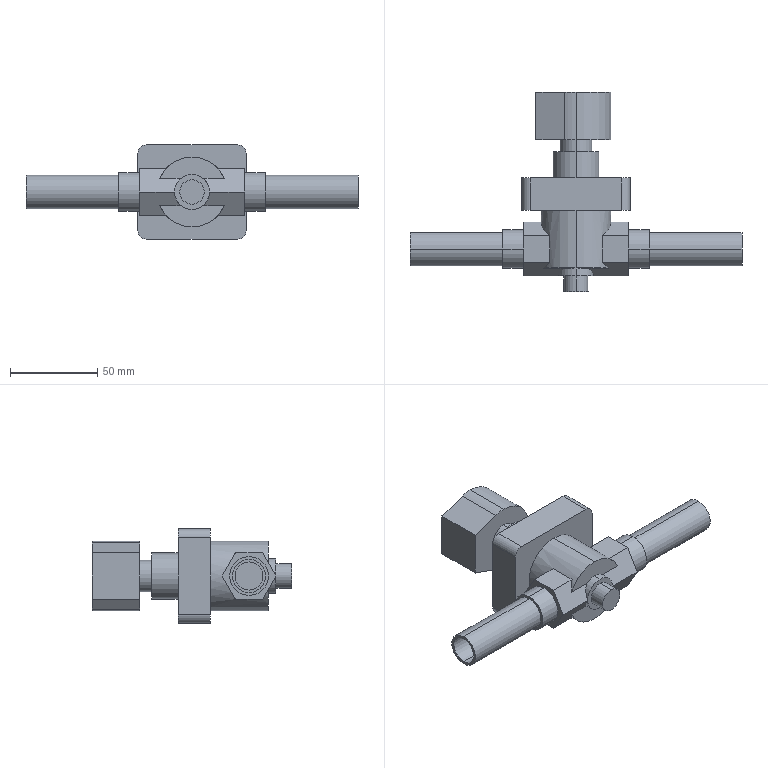Part | STEP file | SEV-1506DYF-three-quarter inlet solenoid valve | 1 solid | 66 faces | box 190 x 114 x 54 mm | volume 186702 mm3 | plane 36 | cylinder 30 | commonest cylinder face diameters 40 x5 10 x4 16.05 x4 19.05 x4 22.2 x4 20 x3